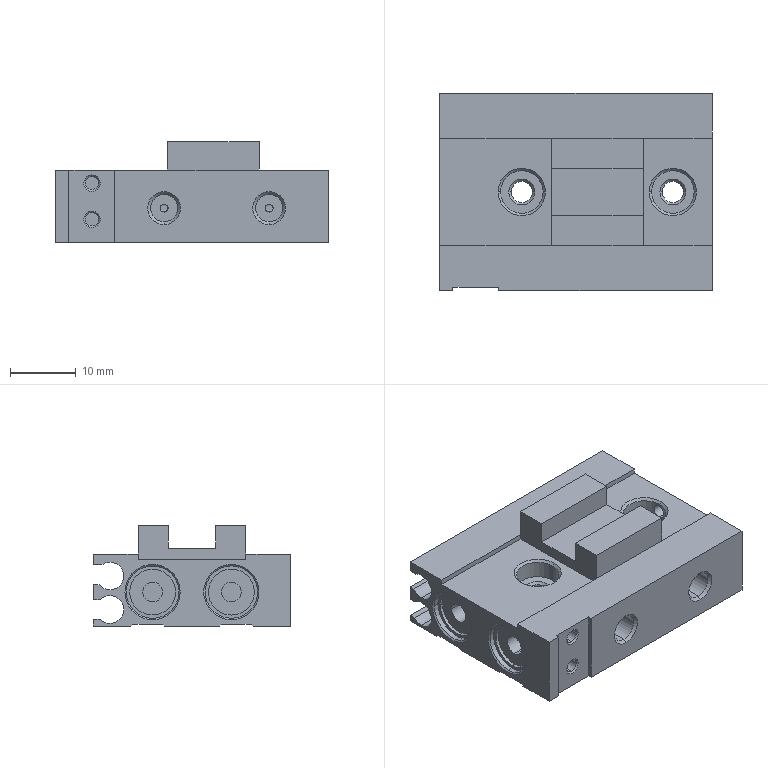Part | STEP file | 11-HLQL6X10-S-0-body-A11 | 1 solid | 167 faces | box 41.5 x 30 x 15.3 mm | volume 10231 mm3 | cylinder 63 | plane 62 | cone 42 | commonest cylinder face diameters 2.013 x12 3 x9 7 x8 8 x8 4.2 x6 1.2 x4